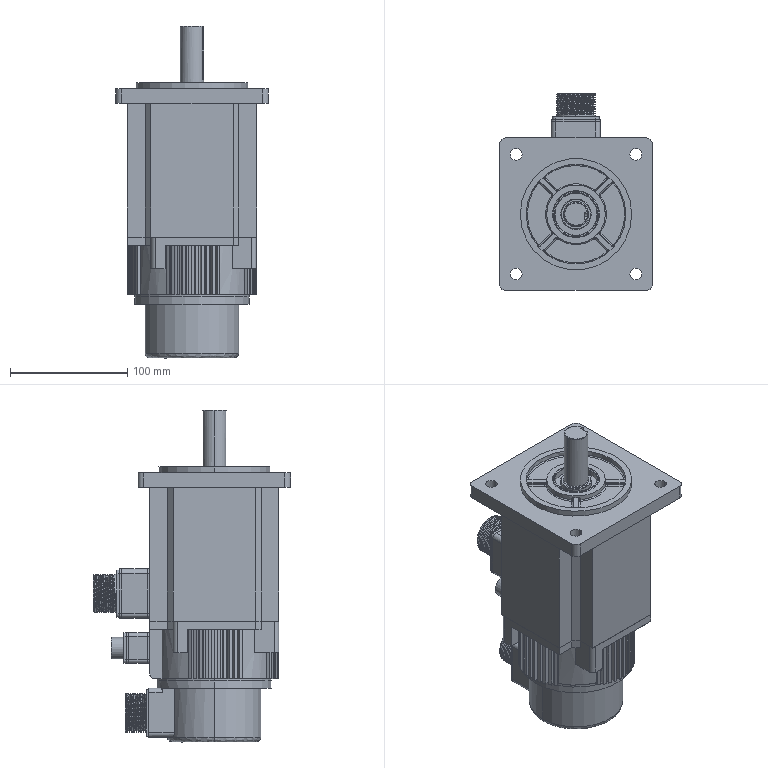Part | STEP file | 110ST-M04030LFBZ | 15 solids | 572 faces | box 130 x 168 x 283 mm | volume 2271146 mm3 | cylinder 259 | plane 227 | cone 47 | spline 39 | commonest cylinder face diameters 33 x52 98 x35 2.5 x24 6 x22 8 x21 4 x20